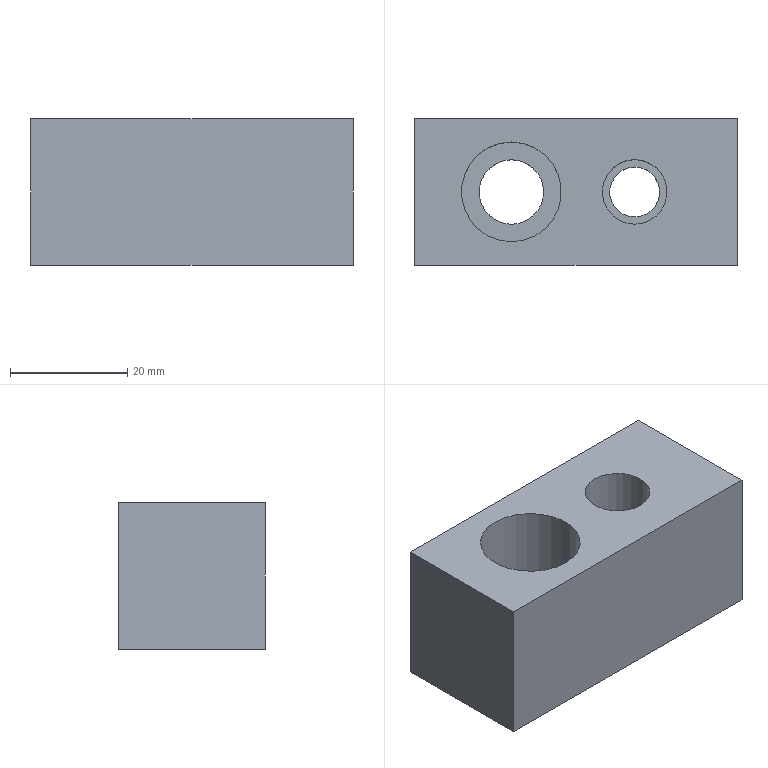Part | STEP file | lll_id4914_x_t | 1 solid | 85 faces | box 55 x 25 x 25 mm | volume 28493 mm3 | plane 67 | other 14 | cylinder 4 | commonest cylinder face diameters 11 x2 8.5 x1 17 x1